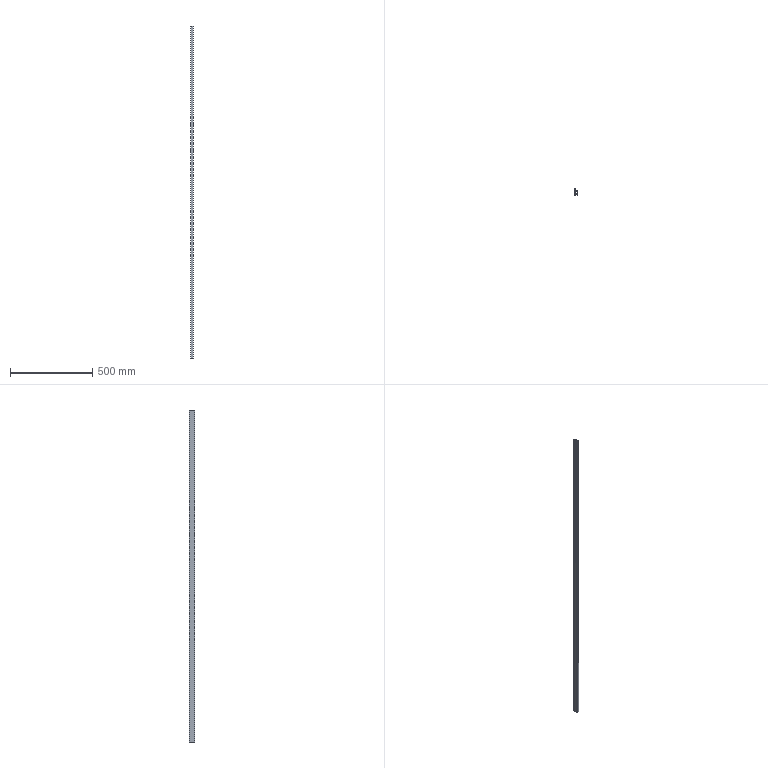Part | 1 solid | 40 faces | box 14.605 x 34.798 x 2016 mm | volume 327940 mm3 | plane 23 | cylinder 17 | commonest cylinder face diameters 0.24 x4 0.2 x3 0.4 x2 0.5 x2 1 x2 1.2 x2
STEP:
#1=CARTESIAN_POINT('',(5.7,32.998,1008.));
#2=VERTEX_POINT('',#1);
#3=CARTESIAN_POINT('',(5.8,32.898,1008.));
#4=VERTEX_POINT('',#3);
#5=CARTESIAN_POINT('',(5.8,32.998,1008.));
#6=DIRECTION('',(0.,0.,1.));
#7=DIRECTION('',(1.,0.,0.));
#8=AXIS2_PLACEMENT_3D('',#5,#6,#7);
#9=CIRCLE('',#8,0.1);
#10=EDGE_CURVE('',#2,#4,#9,.T.);
#11=ORIENTED_EDGE('',*,*,#10,.F.);
#12=CARTESIAN_POINT('',(5.7,32.998,-1008.));
#13=VERTEX_POINT('',#12);
#14=CARTESIAN_POINT('',(5.7,32.998,1008.));
#15=DIRECTION('',(0.,0.,-1.));
#16=VECTOR('',#15,1000.);
#17=LINE('',#14,#16);
#18=EDGE_CURVE('',#2,#13,#17,.T.);
#19=ORIENTED_EDGE('',*,*,#18,.T.);
#20=CARTESIAN_POINT('',(5.8,32.898,-1008.));
#21=VERTEX_POINT('',#20);
#22=CARTESIAN_POINT('',(5.8,32.998,-1008.));
#23=DIRECTION('',(0.,0.,1.));
#24=DIRECTION('',(1.,0.,0.));
#25=AXIS2_PLACEMENT_3D('',#22,#23,#24);
#26=CIRCLE('',#25,0.1);
#27=EDGE_CURVE('',#13,#21,#26,.T.);
#28=ORIENTED_EDGE('',*,*,#27,.T.);
#29=CARTESIAN_POINT('',(5.8,32.898,1008.));
#30=DIRECTION('',(0.,0.,-1.));
#31=VECTOR('',#30,1000.);
#32=LINE('',#29,#31);
#33=EDGE_CURVE('',#4,#21,#32,.T.);
#34=ORIENTED_EDGE('',*,*,#33,.F.);
#35=EDGE_LOOP('',(#11,#19,#28,#34));
#36=FACE_OUTER_BOUND('',#35,.T.);
#37=CARTESIAN_POINT('',(5.8,32.998,1008.));
#38=DIRECTION('',(0.,0.,-1.));
#39=DIRECTION('',(-1.,0.,0.));
#40=AXIS2_PLACEMENT_3D('',#37,#38,#39);
#41=CYLINDRICAL_SURFACE('',#40,0.1);
#42=ADVANCED_FACE('',(#36),#41,.T.);
#43=CARTESIAN_POINT('',(1.75,10.,1008.));
#44=VERTEX_POINT('',#43);
#45=CARTESIAN_POINT('',(2.,10.25,1008.));
#46=VERTEX_POINT('',#45);
#47=CARTESIAN_POINT('',(2.,10.,1008.));
#48=DIRECTION('',(0.,0.,-1.));
#49=DIRECTION('',(1.,0.,0.));
#50=AXIS2_PLACEMENT_3D('',#47,#48,#49);
#51=CIRCLE('',#50,0.25);
#52=EDGE_CURVE('',#44,#46,#51,.T.);
#53=ORIENTED_EDGE('',*,*,#52,.F.);
#54=CARTESIAN_POINT('',(1.75,10.,-1008.));
#55=VERTEX_POINT('',#54);
#56=CARTESIAN_POINT('',(1.75,10.,1008.));
#57=DIRECTION('',(0.,0.,-1.));
#58=VECTOR('',#57,1000.);
#59=LINE('',#56,#58);
#60=EDGE_CURVE('',#44,#55,#59,.T.);
#61=ORIENTED_EDGE('',*,*,#60,.T.);
#62=CARTESIAN_POINT('',(2.,10.25,-1008.));
#63=VERTEX_POINT('',#62);
#64=CARTESIAN_POINT('',(2.,10.,-1008.));
#65=DIRECTION('',(0.,0.,-1.));
#66=DIRECTION('',(1.,0.,0.));
#67=AXIS2_PLACEMENT_3D('',#64,#65,#66);
#68=CIRCLE('',#67,0.25);
#69=EDGE_CURVE('',#55,#63,#68,.T.);
#70=ORIENTED_EDGE('',*,*,#69,.T.);
#71=CARTESIAN_POINT('',(2.,10.25,1008.));
#72=DIRECTION('',(0.,0.,-1.));
#73=VECTOR('',#72,1000.);
#74=LINE('',#71,#73);
#75=EDGE_CURVE('',#46,#63,#74,.T.);
#76=ORIENTED_EDGE('',*,*,#75,.F.);
#77=EDGE_LOOP('',(#53,#61,#70,#76));
#78=FACE_OUTER_BOUND('',#77,.T.);
#79=CARTESIAN_POINT('',(2.,10.,1008.));
#80=DIRECTION('',(0.,0.,-1.));
#81=DIRECTION('',(-1.,0.,0.));
#82=AXIS2_PLACEMENT_3D('',#79,#80,#81);
#83=CYLINDRICAL_SURFACE('',#82,0.25);
#84=ADVANCED_FACE('',(#78),#83,.F.);
#85=CARTESIAN_POINT('',(14.605,7.029,-1008.));
#86=VERTEX_POINT('',#85);
#87=CARTESIAN_POINT('',(14.485,7.149,-1008.));
#88=VERTEX_POINT('',#87);
#89=CARTESIAN_POINT('',(14.485,7.029,-1008.));
#90=DIRECTION('',(0.,0.,1.));
#91=DIRECTION('',(1.,0.,0.));
#92=AXIS2_PLACEMENT_3D('',#89,#90,#91);
#93=CIRCLE('',#92,0.12);
#94=EDGE_CURVE('',#86,#88,#93,.T.);
#95=ORIENTED_EDGE('',*,*,#94,.T.);
#96=CARTESIAN_POINT('',(14.485,7.149,1008.));
#97=VERTEX_POINT('',#96);
#98=CARTESIAN_POINT('',(14.485,7.149,1008.));
#99=DIRECTION('',(0.,0.,-1.));
#100=VECTOR('',#99,1000.);
#101=LINE('',#98,#100);
#102=EDGE_CURVE('',#97,#88,#101,.T.);
#103=ORIENTED_EDGE('',*,*,#102,.F.);
#104=CARTESIAN_POINT('',(14.605,7.029,1008.));
#105=VERTEX_POINT('',#104);
#106=CARTESIAN_POINT('',(14.485,7.029,1008.));
#107=DIRECTION('',(0.,0.,1.));
#108=DIRECTION('',(1.,0.,0.));
#109=AXIS2_PLACEMENT_3D('',#106,#107,#108);
#110=CIRCLE('',#109,0.12);
#111=EDGE_CURVE('',#105,#97,#110,.T.);
#112=ORIENTED_EDGE('',*,*,#111,.F.);
#113=CARTESIAN_POINT('',(14.605,7.029,1008.));
#114=DIRECTION('',(0.,0.,-1.));
#115=VECTOR('',#114,1000.);
#116=LINE('',#113,#115);
#117=EDGE_CURVE('',#105,#86,#116,.T.);
#118=ORIENTED_EDGE('',*,*,#117,.T.);
#119=EDGE_LOOP('',(#95,#103,#112,#118));
#120=FACE_OUTER_BOUND('',#119,.T.);
#121=CARTESIAN_POINT('',(14.485,7.029,1008.));
#122=DIRECTION('',(0.,0.,-1.));
#123=DIRECTION('',(-1.,0.,0.));
#124=AXIS2_PLACEMENT_3D('',#121,#122,#123);
#125=CYLINDRICAL_SURFACE('',#124,0.12);
#126=ADVANCED_FACE('',(#120),#125,.T.);
#127=CARTESIAN_POINT('',(13.705,7.149,-1008.));
#128=VERTEX_POINT('',#127);
#129=CARTESIAN_POINT('',(14.485,7.149,-1008.));
#130=DIRECTION('',(-1.,0.,0.));
#131=VECTOR('',#130,1000.);
#132=LINE('',#129,#131);
#133=EDGE_CURVE('',#88,#128,#132,.T.);
#134=ORIENTED_EDGE('',*,*,#133,.T.);
#135=CARTESIAN_POINT('',(13.705,7.149,1008.));
#136=VERTEX_POINT('',#135);
#137=CARTESIAN_POINT('',(13.705,7.149,1008.));
#138=DIRECTION('',(0.,0.,-1.));
#139=VECTOR('',#138,1000.);
#140=LINE('',#137,#139);
#141=EDGE_CURVE('',#136,#128,#140,.T.);
#142=ORIENTED_EDGE('',*,*,#141,.F.);
#143=CARTESIAN_POINT('',(14.485,7.149,1008.));
#144=DIRECTION('',(-1.,0.,0.));
#145=VECTOR('',#144,1000.);
#146=LINE('',#143,#145);
#147=EDGE_CURVE('',#97,#136,#146,.T.);
#148=ORIENTED_EDGE('',*,*,#147,.F.);
#149=ORIENTED_EDGE('',*,*,#102,.T.);
#150=EDGE_LOOP('',(#134,#142,#148,#149));
#151=FACE_OUTER_BOUND('',#150,.T.);
#152=CARTESIAN_POINT('',(14.485,7.149,1008.));
#153=DIRECTION('',(0.,-1.,0.));
#154=DIRECTION('',(0.,0.,-1.));
#155=AXIS2_PLACEMENT_3D('',#152,#153,#154);
#156=PLANE('',#155);
#157=ADVANCED_FACE('',(#151),#156,.F.);
#158=CARTESIAN_POINT('',(13.105,6.549,-1008.));
#159=VERTEX_POINT('',#158);
#160=CARTESIAN_POINT('',(13.705,6.549,-1008.));
#161=DIRECTION('',(0.,0.,1.));
#162=DIRECTION('',(1.,0.,0.));
#163=AXIS2_PLACEMENT_3D('',#160,#161,#162);
#164=CIRCLE('',#163,0.6);
#165=EDGE_CURVE('',#128,#159,#164,.T.);
#166=ORIENTED_EDGE('',*,*,#165,.T.);
#167=CARTESIAN_POINT('',(13.105,6.549,1008.));
#168=VERTEX_POINT('',#167);
#169=CARTESIAN_POINT('',(13.105,6.549,1008.));
#170=DIRECTION('',(0.,0.,-1.));
#171=VECTOR('',#170,1000.);
#172=LINE('',#169,#171);
#173=EDGE_CURVE('',#168,#159,#172,.T.);
#174=ORIENTED_EDGE('',*,*,#173,.F.);
#175=CARTESIAN_POINT('',(13.705,6.549,1008.));
#176=DIRECTION('',(0.,0.,1.));
#177=DIRECTION('',(1.,0.,0.));
#178=AXIS2_PLACEMENT_3D('',#175,#176,#177);
#179=CIRCLE('',#178,0.6);
#180=EDGE_CURVE('',#136,#168,#179,.T.);
#181=ORIENTED_EDGE('',*,*,#180,.F.);
#182=ORIENTED_EDGE('',*,*,#141,.T.);
#183=EDGE_LOOP('',(#166,#174,#181,#182));
#184=FACE_OUTER_BOUND('',#183,.T.);
#185=CARTESIAN_POINT('',(13.705,6.549,1008.));
#186=DIRECTION('',(0.,0.,-1.));
#187=DIRECTION('',(-1.,0.,0.));
#188=AXIS2_PLACEMENT_3D('',#185,#186,#187);
#189=CYLINDRICAL_SURFACE('',#188,0.6);
#190=ADVANCED_FACE('',(#184),#189,.T.);
#191=CARTESIAN_POINT('',(13.105,2.27,-1008.));
#192=VERTEX_POINT('',#191);
#193=CARTESIAN_POINT('',(13.105,6.549,-1008.));
#194=DIRECTION('',(0.,-1.,0.));
#195=VECTOR('',#194,1000.);
#196=LINE('',#193,#195);
#197=EDGE_CURVE('',#159,#192,#196,.T.);
#198=ORIENTED_EDGE('',*,*,#197,.T.);
#199=CARTESIAN_POINT('',(13.105,2.27,1008.));
#200=VERTEX_POINT('',#199);
#201=CARTESIAN_POINT('',(13.105,2.27,1008.));
#202=DIRECTION('',(0.,0.,-1.));
#203=VECTOR('',#202,1000.);
#204=LINE('',#201,#203);
#205=EDGE_CURVE('',#200,#192,#204,.T.);
#206=ORIENTED_EDGE('',*,*,#205,.F.);
#207=CARTESIAN_POINT('',(13.105,6.549,1008.));
#208=DIRECTION('',(0.,-1.,0.));
#209=VECTOR('',#208,1000.);
#210=LINE('',#207,#209);
#211=EDGE_CURVE('',#168,#200,#210,.T.);
#212=ORIENTED_EDGE('',*,*,#211,.F.);
#213=ORIENTED_EDGE('',*,*,#173,.T.);
#214=EDGE_LOOP('',(#198,#206,#212,#213));
#215=FACE_OUTER_BOUND('',#214,.T.);
#216=CARTESIAN_POINT('',(13.105,6.549,1008.));
#217=DIRECTION('',(1.,0.,0.));
#218=DIRECTION('',(0.,0.,-1.));
#219=AXIS2_PLACEMENT_3D('',#216,#217,#218);
#220=PLANE('',#219);
#221=ADVANCED_FACE('',(#215),#220,.F.);
#222=CARTESIAN_POINT('',(12.985,2.15,-1008.));
#223=VERTEX_POINT('',#222);
#224=CARTESIAN_POINT('',(12.985,2.27,-1008.));
#225=DIRECTION('',(0.,0.,-1.));
#226=DIRECTION('',(1.,0.,0.));
#227=AXIS2_PLACEMENT_3D('',#224,#225,#226);
#228=CIRCLE('',#227,0.12);
#229=EDGE_CURVE('',#192,#223,#228,.T.);
#230=ORIENTED_EDGE('',*,*,#229,.T.);
#231=CARTESIAN_POINT('',(12.985,2.15,1008.));
#232=VERTEX_POINT('',#231);
#233=CARTESIAN_POINT('',(12.985,2.15,1008.));
#234=DIRECTION('',(0.,0.,-1.));
#235=VECTOR('',#234,1000.);
#236=LINE('',#233,#235);
#237=EDGE_CURVE('',#232,#223,#236,.T.);
#238=ORIENTED_EDGE('',*,*,#237,.F.);
#239=CARTESIAN_POINT('',(12.985,2.27,1008.));
#240=DIRECTION('',(0.,0.,-1.));
#241=DIRECTION('',(1.,0.,0.));
#242=AXIS2_PLACEMENT_3D('',#239,#240,#241);
#243=CIRCLE('',#242,0.12);
#244=EDGE_CURVE('',#200,#232,#243,.T.);
#245=ORIENTED_EDGE('',*,*,#244,.F.);
#246=ORIENTED_EDGE('',*,*,#205,.T.);
#247=EDGE_LOOP('',(#230,#238,#245,#246));
#248=FACE_OUTER_BOUND('',#247,.T.);
#249=CARTESIAN_POINT('',(12.985,2.27,1008.));
#250=DIRECTION('',(0.,0.,-1.));
#251=DIRECTION('',(-1.,0.,0.));
#252=AXIS2_PLACEMENT_3D('',#249,#250,#251);
#253=CYLINDRICAL_SURFACE('',#252,0.12);
#254=ADVANCED_FACE('',(#248),#253,.F.);
#255=CARTESIAN_POINT('',(2.5,2.15,-1008.));
#256=VERTEX_POINT('',#255);
#257=CARTESIAN_POINT('',(12.985,2.15,-1008.));
#258=DIRECTION('',(-1.,0.00001466,0.));
#259=VECTOR('',#258,1000.);
#260=LINE('',#257,#259);
#261=EDGE_CURVE('',#223,#256,#260,.T.);
#262=ORIENTED_EDGE('',*,*,#261,.T.);
#263=CARTESIAN_POINT('',(2.5,2.15,1008.));
#264=VERTEX_POINT('',#263);
#265=CARTESIAN_POINT('',(2.5,2.15,1008.));
#266=DIRECTION('',(0.,0.,-1.));
#267=VECTOR('',#266,1000.);
#268=LINE('',#265,#267);
#269=EDGE_CURVE('',#264,#256,#268,.T.);
#270=ORIENTED_EDGE('',*,*,#269,.F.);
#271=CARTESIAN_POINT('',(12.985,2.15,1008.));
#272=DIRECTION('',(-1.,0.00001466,0.));
#273=VECTOR('',#272,1000.);
#274=LINE('',#271,#273);
#275=EDGE_CURVE('',#232,#264,#274,.T.);
#276=ORIENTED_EDGE('',*,*,#275,.F.);
#277=ORIENTED_EDGE('',*,*,#237,.T.);
#278=EDGE_LOOP('',(#262,#270,#276,#277));
#279=FACE_OUTER_BOUND('',#278,.T.);
#280=CARTESIAN_POINT('',(12.985,2.15,1008.));
#281=DIRECTION('',(-0.00001466,-1.,0.));
#282=DIRECTION('',(1.,-0.00001466,0.));
#283=AXIS2_PLACEMENT_3D('',#280,#281,#282);
#284=PLANE('',#283);
#285=ADVANCED_FACE('',(#279),#284,.F.);
#286=CARTESIAN_POINT('',(2.,2.65,-1008.));
#287=VERTEX_POINT('',#286);
#288=CARTESIAN_POINT('',(2.5,2.65,-1008.));
#289=DIRECTION('',(0.,0.,-1.));
#290=DIRECTION('',(1.,0.,0.));
#291=AXIS2_PLACEMENT_3D('',#288,#289,#290);
#292=CIRCLE('',#291,0.5);
#293=EDGE_CURVE('',#256,#287,#292,.T.);
#294=ORIENTED_EDGE('',*,*,#293,.T.);
#295=CARTESIAN_POINT('',(2.,2.65,1008.));
#296=VERTEX_POINT('',#295);
#297=CARTESIAN_POINT('',(2.,2.65,1008.));
#298=DIRECTION('',(0.,0.,-1.));
#299=VECTOR('',#298,1000.);
#300=LINE('',#297,#299);
#301=EDGE_CURVE('',#296,#287,#300,.T.);
#302=ORIENTED_EDGE('',*,*,#301,.F.);
#303=CARTESIAN_POINT('',(2.5,2.65,1008.));
#304=DIRECTION('',(0.,0.,-1.));
#305=DIRECTION('',(1.,0.,0.));
#306=AXIS2_PLACEMENT_3D('',#303,#304,#305);
#307=CIRCLE('',#306,0.5);
#308=EDGE_CURVE('',#264,#296,#307,.T.);
#309=ORIENTED_EDGE('',*,*,#308,.F.);
#310=ORIENTED_EDGE('',*,*,#269,.T.);
#311=EDGE_LOOP('',(#294,#302,#309,#310));
#312=FACE_OUTER_BOUND('',#311,.T.);
#313=CARTESIAN_POINT('',(2.5,2.65,1008.));
#314=DIRECTION('',(0.,0.,-1.));
#315=DIRECTION('',(-1.,0.,0.));
#316=AXIS2_PLACEMENT_3D('',#313,#314,#315);
#317=CYLINDRICAL_SURFACE('',#316,0.5);
#318=ADVANCED_FACE('',(#312),#317,.F.);
#319=CARTESIAN_POINT('',(2.,9.75,-1008.));
#320=VERTEX_POINT('',#319);
#321=CARTESIAN_POINT('',(2.,2.65,-1008.));
#322=DIRECTION('',(0.,1.,0.));
#323=VECTOR('',#322,1000.);
#324=LINE('',#321,#323);
#325=EDGE_CURVE('',#287,#320,#324,.T.);
#326=ORIENTED_EDGE('',*,*,#325,.T.);
#327=CARTESIAN_POINT('',(2.,9.75,1008.));
#328=VERTEX_POINT('',#327);
#329=CARTESIAN_POINT('',(2.,9.75,1008.));
#330=DIRECTION('',(0.,0.,-1.));
#331=VECTOR('',#330,1000.);
#332=LINE('',#329,#331);
#333=EDGE_CURVE('',#328,#320,#332,.T.);
#334=ORIENTED_EDGE('',*,*,#333,.F.);
#335=CARTESIAN_POINT('',(2.,2.65,1008.));
#336=DIRECTION('',(0.,1.,0.));
#337=VECTOR('',#336,1000.);
#338=LINE('',#335,#337);
#339=EDGE_CURVE('',#296,#328,#338,.T.);
#340=ORIENTED_EDGE('',*,*,#339,.F.);
#341=ORIENTED_EDGE('',*,*,#301,.T.);
#342=EDGE_LOOP('',(#326,#334,#340,#341));
#343=FACE_OUTER_BOUND('',#342,.T.);
#344=CARTESIAN_POINT('',(2.,2.65,1008.));
#345=DIRECTION('',(-1.,0.,0.));
#346=DIRECTION('',(0.,0.,1.));
#347=AXIS2_PLACEMENT_3D('',#344,#345,#346);
#348=PLANE('',#347);
#349=ADVANCED_FACE('',(#343),#348,.F.);
#350=ORIENTED_EDGE('',*,*,#60,.F.);
#351=CARTESIAN_POINT('',(2.,10.,1008.));
#352=DIRECTION('',(0.,0.,-1.));
#353=DIRECTION('',(1.,0.,0.));
#354=AXIS2_PLACEMENT_3D('',#351,#352,#353);
#355=CIRCLE('',#354,0.25);
#356=EDGE_CURVE('',#328,#44,#355,.T.);
#357=ORIENTED_EDGE('',*,*,#356,.F.);
#358=ORIENTED_EDGE('',*,*,#333,.T.);
#359=CARTESIAN_POINT('',(2.,10.,-1008.));
#360=DIRECTION('',(0.,0.,-1.));
#361=DIRECTION('',(1.,0.,0.));
#362=AXIS2_PLACEMENT_3D('',#359,#360,#361);
#363=CIRCLE('',#362,0.25);
#364=EDGE_CURVE('',#320,#55,#363,.T.);
#365=ORIENTED_EDGE('',*,*,#364,.T.);
#366=EDGE_LOOP('',(#350,#357,#358,#365));
#367=FACE_OUTER_BOUND('',#366,.T.);
#368=CARTESIAN_POINT('',(2.,10.,1008.));
#369=DIRECTION('',(0.,0.,-1.));
#370=DIRECTION('',(-1.,0.,0.));
#371=AXIS2_PLACEMENT_3D('',#368,#369,#370);
#372=CYLINDRICAL_SURFACE('',#371,0.25);
#373=ADVANCED_FACE('',(#367),#372,.F.);
#374=CARTESIAN_POINT('',(2.,17.35,-1008.));
#375=VERTEX_POINT('',#374);
#376=CARTESIAN_POINT('',(2.,10.25,-1008.));
#377=DIRECTION('',(0.,1.,0.));
#378=VECTOR('',#377,1000.);
#379=LINE('',#376,#378);
#380=EDGE_CURVE('',#63,#375,#379,.T.);
#381=ORIENTED_EDGE('',*,*,#380,.T.);
#382=CARTESIAN_POINT('',(2.,17.35,1008.));
#383=VERTEX_POINT('',#382);
#384=CARTESIAN_POINT('',(2.,17.35,1008.));
#385=DIRECTION('',(0.,0.,-1.));
#386=VECTOR('',#385,1000.);
#387=LINE('',#384,#386);
#388=EDGE_CURVE('',#383,#375,#387,.T.);
#389=ORIENTED_EDGE('',*,*,#388,.F.);
#390=CARTESIAN_POINT('',(2.,10.25,1008.));
#391=DIRECTION('',(0.,1.,0.));
#392=VECTOR('',#391,1000.);
#393=LINE('',#390,#392);
#394=EDGE_CURVE('',#46,#383,#393,.T.);
#395=ORIENTED_EDGE('',*,*,#394,.F.);
#396=ORIENTED_EDGE('',*,*,#75,.T.);
#397=EDGE_LOOP('',(#381,#389,#395,#396));
#398=FACE_OUTER_BOUND('',#397,.T.);
#399=CARTESIAN_POINT('',(2.,10.25,1008.));
#400=DIRECTION('',(-1.,0.,0.));
#401=DIRECTION('',(0.,0.,1.));
#402=AXIS2_PLACEMENT_3D('',#399,#400,#401);
#403=PLANE('',#402);
#404=ADVANCED_FACE('',(#398),#403,.F.);
#405=CARTESIAN_POINT('',(2.5,17.85,-1008.));
#406=VERTEX_POINT('',#405);
#407=CARTESIAN_POINT('',(2.5,17.35,-1008.));
#408=DIRECTION('',(0.,0.,-1.));
#409=DIRECTION('',(1.,0.,0.));
#410=AXIS2_PLACEMENT_3D('',#407,#408,#409);
#411=CIRCLE('',#410,0.5);
#412=EDGE_CURVE('',#375,#406,#411,.T.);
#413=ORIENTED_EDGE('',*,*,#412,.T.);
#414=CARTESIAN_POINT('',(2.5,17.85,1008.));
#415=VERTEX_POINT('',#414);
#416=CARTESIAN_POINT('',(2.5,17.85,1008.));
#417=DIRECTION('',(0.,0.,-1.));
#418=VECTOR('',#417,1000.);
#419=LINE('',#416,#418);
#420=EDGE_CURVE('',#415,#406,#419,.T.);
#421=ORIENTED_EDGE('',*,*,#420,.F.);
#422=CARTESIAN_POINT('',(2.5,17.35,1008.));
#423=DIRECTION('',(0.,0.,-1.));
#424=DIRECTION('',(1.,0.,0.));
#425=AXIS2_PLACEMENT_3D('',#422,#423,#424);
#426=CIRCLE('',#425,0.5);
#427=EDGE_CURVE('',#383,#415,#426,.T.);
#428=ORIENTED_EDGE('',*,*,#427,.F.);
#429=ORIENTED_EDGE('',*,*,#388,.T.);
#430=EDGE_LOOP('',(#413,#421,#428,#429));
#431=FACE_OUTER_BOUND('',#430,.T.);
#432=CARTESIAN_POINT('',(2.5,17.35,1008.));
#433=DIRECTION('',(0.,0.,-1.));
#434=DIRECTION('',(-1.,0.,0.));
#435=AXIS2_PLACEMENT_3D('',#432,#433,#434);
#436=CYLINDRICAL_SURFACE('',#435,0.5);
#437=ADVANCED_FACE('',(#431),#436,.F.);
#438=CARTESIAN_POINT('',(14.604,17.85,-1008.));
#439=VERTEX_POINT('',#438);
#440=CARTESIAN_POINT('',(2.5,17.85,-1008.));
#441=DIRECTION('',(1.,0.,0.));
#442=VECTOR('',#441,1000.);
#443=LINE('',#440,#442);
#444=EDGE_CURVE('',#406,#439,#443,.T.);
#445=ORIENTED_EDGE('',*,*,#444,.T.);
#446=CARTESIAN_POINT('',(14.604,17.85,1008.));
#447=VERTEX_POINT('',#446);
#448=CARTESIAN_POINT('',(14.604,17.85,1008.));
#449=DIRECTION('',(0.,0.,-1.));
#450=VECTOR('',#449,1000.);
#451=LINE('',#448,#450);
#452=EDGE_CURVE('',#447,#439,#451,.T.);
#453=ORIENTED_EDGE('',*,*,#452,.F.);
#454=CARTESIAN_POINT('',(2.5,17.85,1008.));
#455=DIRECTION('',(1.,0.,0.));
#456=VECTOR('',#455,1000.);
#457=LINE('',#454,#456);
#458=EDGE_CURVE('',#415,#447,#457,.T.);
#459=ORIENTED_EDGE('',*,*,#458,.F.);
#460=ORIENTED_EDGE('',*,*,#420,.T.);
#461=EDGE_LOOP('',(#445,#453,#459,#460));
#462=FACE_OUTER_BOUND('',#461,.T.);
#463=CARTESIAN_POINT('',(2.5,17.85,1008.));
#464=DIRECTION('',(0.,1.,0.));
#465=DIRECTION('',(0.,0.,1.));
#466=AXIS2_PLACEMENT_3D('',#463,#464,#465);
#467=PLANE('',#466);
#468=ADVANCED_FACE('',(#462),#467,.F.);
#469=CARTESIAN_POINT('',(14.604,23.83,-1008.));
#470=VERTEX_POINT('',#469);
#471=CARTESIAN_POINT('',(14.604,17.85,-1008.));
#472=DIRECTION('',(0.,1.,0.));
#473=VECTOR('',#472,1000.);
#474=LINE('',#471,#473);
#475=EDGE_CURVE('',#439,#470,#474,.T.);
#476=ORIENTED_EDGE('',*,*,#475,.T.);
#477=CARTESIAN_POINT('',(14.604,23.83,1008.));
#478=VERTEX_POINT('',#477);
#479=CARTESIAN_POINT('',(14.604,23.83,1008.));
#480=DIRECTION('',(0.,0.,-1.));
#481=VECTOR('',#480,1000.);
#482=LINE('',#479,#481);
#483=EDGE_CURVE('',#478,#470,#482,.T.);
#484=ORIENTED_EDGE('',*,*,#483,.F.);
#485=CARTESIAN_POINT('',(14.604,17.85,1008.));
#486=DIRECTION('',(0.,1.,0.));
#487=VECTOR('',#486,1000.);
#488=LINE('',#485,#487);
#489=EDGE_CURVE('',#447,#478,#488,.T.);
#490=ORIENTED_EDGE('',*,*,#489,.F.);
#491=ORIENTED_EDGE('',*,*,#452,.T.);
#492=EDGE_LOOP('',(#476,#484,#490,#491));
#493=FACE_OUTER_BOUND('',#492,.T.);
#494=CARTESIAN_POINT('',(14.604,17.85,1008.));
#495=DIRECTION('',(-1.,0.,0.));
#496=DIRECTION('',(0.,0.,1.));
#497=AXIS2_PLACEMENT_3D('',#494,#495,#496);
#498=PLANE('',#497);
#499=ADVANCED_FACE('',(#493),#498,.F.);
#500=CARTESIAN_POINT('',(14.484,23.95,-1008.));
#501=VERTEX_POINT('',#500);
#502=CARTESIAN_POINT('',(14.484,23.83,-1008.));
#503=DIRECTION('',(0.,0.,1.));
#504=DIRECTION('',(1.,0.,0.));
#505=AXIS2_PLACEMENT_3D('',#502,#503,#504);
#506=CIRCLE('',#505,0.12);
#507=EDGE_CURVE('',#470,#501,#506,.T.);
#508=ORIENTED_EDGE('',*,*,#507,.T.);
#509=CARTESIAN_POINT('',(14.484,23.95,1008.));
#510=VERTEX_POINT('',#509);
#511=CARTESIAN_POINT('',(14.484,23.95,1008.));
#512=DIRECTION('',(0.,0.,-1.));
#513=VECTOR('',#512,1000.);
#514=LINE('',#511,#513);
#515=EDGE_CURVE('',#510,#501,#514,.T.);
#516=ORIENTED_EDGE('',*,*,#515,.F.);
#517=CARTESIAN_POINT('',(14.484,23.83,1008.));
#518=DIRECTION('',(0.,0.,1.));
#519=DIRECTION('',(1.,0.,0.));
#520=AXIS2_PLACEMENT_3D('',#517,#518,#519);
#521=CIRCLE('',#520,0.12);
#522=EDGE_CURVE('',#478,#510,#521,.T.);
#523=ORIENTED_EDGE('',*,*,#522,.F.);
#524=ORIENTED_EDGE('',*,*,#483,.T.);
#525=EDGE_LOOP('',(#508,#516,#523,#524));
#526=FACE_OUTER_BOUND('',#525,.T.);
#527=CARTESIAN_POINT('',(14.484,23.83,1008.));
#528=DIRECTION('',(0.,0.,-1.));
#529=DIRECTION('',(-1.,0.,0.));
#530=AXIS2_PLACEMENT_3D('',#527,#528,#529);
#531=CYLINDRICAL_SURFACE('',#530,0.12);
#532=ADVANCED_FACE('',(#526),#531,.T.);
#533=CARTESIAN_POINT('',(13.704,23.95,-1008.));
#534=VERTEX_POINT('',#533);
#535=CARTESIAN_POINT('',(14.484,23.95,-1008.));
#536=DIRECTION('',(-1.,0.,0.));
#537=VECTOR('',#536,1000.);
#538=LINE('',#535,#537);
#539=EDGE_CURVE('',#501,#534,#538,.T.);
#540=ORIENTED_EDGE('',*,*,#539,.T.);
#541=CARTESIAN_POINT('',(13.704,23.95,1008.));
#542=VERTEX_POINT('',#541);
#543=CARTESIAN_POINT('',(13.704,23.95,1008.));
#544=DIRECTION('',(0.,0.,-1.));
#545=VECTOR('',#544,1000.);
#546=LINE('',#543,#545);
#547=EDGE_CURVE('',#542,#534,#546,.T.);
#548=ORIENTED_EDGE('',*,*,#547,.F.);
#549=CARTESIAN_POINT('',(14.484,23.95,1008.));
#550=DIRECTION('',(-1.,0.,0.));
#551=VECTOR('',#550,1000.);
#552=LINE('',#549,#551);
#553=EDGE_CURVE('',#510,#542,#552,.T.);
#554=ORIENTED_EDGE('',*,*,#553,.F.);
#555=ORIENTED_EDGE('',*,*,#515,.T.);
#556=EDGE_LOOP('',(#540,#548,#554,#555));
#557=FACE_OUTER_BOUND('',#556,.T.);
#558=CARTESIAN_POINT('',(14.484,23.95,1008.));
#559=DIRECTION('',(0.,-1.,0.));
#560=DIRECTION('',(0.,0.,-1.));
#561=AXIS2_PLACEMENT_3D('',#558,#559,#560);
#562=PLANE('',#561);
#563=ADVANCED_FACE('',(#557),#562,.F.);
#564=CARTESIAN_POINT('',(13.104,23.35,-1008.));
#565=VERTEX_POINT('',#564);
#566=CARTESIAN_POINT('',(13.704,23.35,-1008.));
#567=DIRECTION('',(0.,0.,1.));
#568=DIRECTION('',(1.,0.,0.));
#569=AXIS2_PLACEMENT_3D('',#566,#567,#568);
#570=CIRCLE('',#569,0.6);
#571=EDGE_CURVE('',#534,#565,#570,.T.);
#572=ORIENTED_EDGE('',*,*,#571,.T.);
#573=CARTESIAN_POINT('',(13.104,23.35,1008.));
#574=VERTEX_POINT('',#573);
#575=CARTESIAN_POINT('',(13.104,23.35,1008.));
#576=DIRECTION('',(0.,0.,-1.));
#577=VECTOR('',#576,1000.);
#578=LINE('',#575,#577);
#579=EDGE_CURVE('',#574,#565,#578,.T.);
#580=ORIENTED_EDGE('',*,*,#579,.F.);
#581=CARTESIAN_POINT('',(13.704,23.35,1008.));
#582=DIRECTION('',(0.,0.,1.));
#583=DIRECTION('',(1.,0.,0.));
#584=AXIS2_PLACEMENT_3D('',#581,#582,#583);
#585=CIRCLE('',#584,0.6);
#586=EDGE_CURVE('',#542,#574,#585,.T.);
#587=ORIENTED_EDGE('',*,*,#586,.F.);
#588=ORIENTED_EDGE('',*,*,#547,.T.);
#589=EDGE_LOOP('',(#572,#580,#587,#588));
#590=FACE_OUTER_BOUND('',#589,.T.);
#591=CARTESIAN_POINT('',(13.704,23.35,1008.));
#592=DIRECTION('',(0.,0.,-1.));
#593=DIRECTION('',(-1.,0.,0.));
#594=AXIS2_PLACEMENT_3D('',#591,#592,#593);
#595=CYLINDRICAL_SURFACE('',#594,0.6);
#596=ADVANCED_FACE('',(#590),#595,.T.);
#597=CARTESIAN_POINT('',(13.104,19.47,-1008.));
#598=VERTEX_POINT('',#597);
#599=CARTESIAN_POINT('',(13.104,23.35,-1008.));
#600=DIRECTION('',(0.,-1.,0.));
#601=VECTOR('',#600,1000.);
#602=LINE('',#599,#601);
#603=EDGE_CURVE('',#565,#598,#602,.T.);
#604=ORIENTED_EDGE('',*,*,#603,.T.);
#605=CARTESIAN_POINT('',(13.104,19.47,1008.));
#606=VERTEX_POINT('',#605);
#607=CARTESIAN_POINT('',(13.104,19.47,1008.));
#608=DIRECTION('',(0.,0.,-1.));
#609=VECTOR('',#608,1000.);
#610=LINE('',#607,#609);
#611=EDGE_CURVE('',#606,#598,#610,.T.);
#612=ORIENTED_EDGE('',*,*,#611,.F.);
#613=CARTESIAN_POINT('',(13.104,23.35,1008.));
#614=DIRECTION('',(0.,-1.,0.));
#615=VECTOR('',#614,1000.);
#616=LINE('',#613,#615);
#617=EDGE_CURVE('',#574,#606,#616,.T.);
#618=ORIENTED_EDGE('',*,*,#617,.F.);
#619=ORIENTED_EDGE('',*,*,#579,.T.);
#620=EDGE_LOOP('',(#604,#612,#618,#619));
#621=FACE_OUTER_BOUND('',#620,.T.);
#622=CARTESIAN_POINT('',(13.104,23.35,1008.));
#623=DIRECTION('',(1.,0.,0.));
#624=DIRECTION('',(0.,0.,-1.));
#625=AXIS2_PLACEMENT_3D('',#622,#623,#624);
#626=PLANE('',#625);
#627=ADVANCED_FACE('',(#621),#626,.F.);
#628=CARTESIAN_POINT('',(12.984,19.35,-1008.));
#629=VERTEX_POINT('',#628);
#630=CARTESIAN_POINT('',(12.984,19.47,-1008.));
#631=DIRECTION('',(0.,0.,-1.));
#632=DIRECTION('',(1.,0.,0.));
#633=AXIS2_PLACEMENT_3D('',#630,#631,#632);
#634=CIRCLE('',#633,0.12);
#635=EDGE_CURVE('',#598,#629,#634,.T.);
#636=ORIENTED_EDGE('',*,*,#635,.T.);
#637=CARTESIAN_POINT('',(12.984,19.35,1008.));
#638=VERTEX_POINT('',#637);
#639=CARTESIAN_POINT('',(12.984,19.35,1008.));
#640=DIRECTION('',(0.,0.,-1.));
#641=VECTOR('',#640,1000.);
#642=LINE('',#639,#641);
#643=EDGE_CURVE('',#638,#629,#642,.T.);
#644=ORIENTED_EDGE('',*,*,#643,.F.);
#645=CARTESIAN_POINT('',(12.984,19.47,1008.));
#646=DIRECTION('',(0.,0.,-1.));
#647=DIRECTION('',(1.,0.,0.));
#648=AXIS2_PLACEMENT_3D('',#645,#646,#647);
#649=CIRCLE('',#648,0.12);
#650=EDGE_CURVE('',#606,#638,#649,.T.);
#651=ORIENTED_EDGE('',*,*,#650,.F.);
#652=ORIENTED_EDGE('',*,*,#611,.T.);
#653=EDGE_LOOP('',(#636,#644,#651,#652));
#654=FACE_OUTER_BOUND('',#653,.T.);
#655=CARTESIAN_POINT('',(12.984,19.47,1008.));
#656=DIRECTION('',(0.,0.,-1.));
#657=DIRECTION('',(-1.,0.,0.));
#658=AXIS2_PLACEMENT_3D('',#655,#656,#657);
#659=CYLINDRICAL_SURFACE('',#658,0.12);
#660=ADVANCED_FACE('',(#654),#659,.F.);
#661=CARTESIAN_POINT('',(7.2,19.35,-1008.));
#662=VERTEX_POINT('',#661);
#663=CARTESIAN_POINT('',(12.984,19.35,-1008.));
#664=DIRECTION('',(-1.,0.,0.));
#665=VECTOR('',#664,1000.);
#666=LINE('',#663,#665);
#667=EDGE_CURVE('',#629,#662,#666,.T.);
#668=ORIENTED_EDGE('',*,*,#667,.T.);
#669=CARTESIAN_POINT('',(7.2,19.35,1008.));
#670=VERTEX_POINT('',#669);
#671=CARTESIAN_POINT('',(7.2,19.35,1008.));
#672=DIRECTION('',(0.,0.,-1.));
#673=VECTOR('',#672,1000.);
#674=LINE('',#671,#673);
#675=EDGE_CURVE('',#670,#662,#674,.T.);
#676=ORIENTED_EDGE('',*,*,#675,.F.);
#677=CARTESIAN_POINT('',(12.984,19.35,1008.));
#678=DIRECTION('',(-1.,0.,0.));
#679=VECTOR('',#678,1000.);
#680=LINE('',#677,#679);
#681=EDGE_CURVE('',#638,#670,#680,.T.);
#682=ORIENTED_EDGE('',*,*,#681,.F.);
#683=ORIENTED_EDGE('',*,*,#643,.T.);
#684=EDGE_LOOP('',(#668,#676,#682,#683));
#685=FACE_OUTER_BOUND('',#684,.T.);
#686=CARTESIAN_POINT('',(12.984,19.35,1008.));
#687=DIRECTION('',(0.,-1.,0.));
#688=DIRECTION('',(0.,0.,-1.));
#689=AXIS2_PLACEMENT_3D('',#686,#687,#688);
#690=PLANE('',#689);
#691=ADVANCED_FACE('',(#685),#690,.F.);
#692=CARTESIAN_POINT('',(7.2,34.798,-1008.));
#693=VERTEX_POINT('',#692);
#694=CARTESIAN_POINT('',(7.2,19.35,-1008.));
#695=DIRECTION('',(0.,1.,0.));
#696=VECTOR('',#695,1000.);
#697=LINE('',#694,#696);
#698=EDGE_CURVE('',#662,#693,#697,.T.);
#699=ORIENTED_EDGE('',*,*,#698,.T.);
#700=CARTESIAN_POINT('',(7.2,34.798,1008.));
#701=VERTEX_POINT('',#700);
#702=CARTESIAN_POINT('',(7.2,34.798,1008.));
#703=DIRECTION('',(0.,0.,-1.));
#704=VECTOR('',#703,1000.);
#705=LINE('',#702,#704);
#706=EDGE_CURVE('',#701,#693,#705,.T.);
#707=ORIENTED_EDGE('',*,*,#706,.F.);
#708=CARTESIAN_POINT('',(7.2,19.35,1008.));
#709=DIRECTION('',(0.,1.,0.));
#710=VECTOR('',#709,1000.);
#711=LINE('',#708,#710);
#712=EDGE_CURVE('',#670,#701,#711,.T.);
#713=ORIENTED_EDGE('',*,*,#712,.F.);
#714=ORIENTED_EDGE('',*,*,#675,.T.);
#715=EDGE_LOOP('',(#699,#707,#713,#714));
#716=FACE_OUTER_BOUND('',#715,.T.);
#717=CARTESIAN_POINT('',(7.2,19.35,1008.));
#718=DIRECTION('',(-1.,0.,0.));
#719=DIRECTION('',(0.,0.,1.));
#720=AXIS2_PLACEMENT_3D('',#717,#718,#719);
#721=PLANE('',#720);
#722=ADVANCED_FACE('',(#716),#721,.F.);
#723=CARTESIAN_POINT('',(6.,34.798,-1008.));
#724=VERTEX_POINT('',#723);
#725=CARTESIAN_POINT('',(7.2,34.798,-1008.));
#726=DIRECTION('',(-1.,0.,0.));
#727=VECTOR('',#726,1000.);
#728=LINE('',#725,#727);
#729=EDGE_CURVE('',#693,#724,#728,.T.);
#730=ORIENTED_EDGE('',*,*,#729,.T.);
#731=CARTESIAN_POINT('',(6.,34.798,1008.));
#732=VERTEX_POINT('',#731);
#733=CARTESIAN_POINT('',(6.,34.798,1008.));
#734=DIRECTION('',(0.,0.,-1.));
#735=VECTOR('',#734,1000.);
#736=LINE('',#733,#735);
#737=EDGE_CURVE('',#732,#724,#736,.T.);
#738=ORIENTED_EDGE('',*,*,#737,.F.);
#739=CARTESIAN_POINT('',(7.2,34.798,1008.));
#740=DIRECTION('',(-1.,0.,0.));
#741=VECTOR('',#740,1000.);
#742=LINE('',#739,#741);
#743=EDGE_CURVE('',#701,#732,#742,.T.);
#744=ORIENTED_EDGE('',*,*,#743,.F.);
#745=ORIENTED_EDGE('',*,*,#706,.T.);
#746=EDGE_LOOP('',(#730,#738,#744,#745));
#747=FACE_OUTER_BOUND('',#746,.T.);
#748=CARTESIAN_POINT('',(7.2,34.798,1008.));
#749=DIRECTION('',(0.,-1.,0.));
#750=DIRECTION('',(0.,0.,-1.));
#751=AXIS2_PLACEMENT_3D('',#748,#749,#750);
#752=PLANE('',#751);
#753=ADVANCED_FACE('',(#747),#752,.F.);
#754=CARTESIAN_POINT('',(5.8,34.598,-1008.));
#755=VERTEX_POINT('',#754);
#756=CARTESIAN_POINT('',(6.,34.598,-1008.));
#757=DIRECTION('',(0.,0.,1.));
#758=DIRECTION('',(1.,0.,0.));
#759=AXIS2_PLACEMENT_3D('',#756,#757,#758);
#760=CIRCLE('',#759,0.2);
#761=EDGE_CURVE('',#724,#755,#760,.T.);
#762=ORIENTED_EDGE('',*,*,#761,.T.);
#763=CARTESIAN_POINT('',(5.8,34.598,1008.));
#764=VERTEX_POINT('',#763);
#765=CARTESIAN_POINT('',(5.8,34.598,1008.));
#766=DIRECTION('',(0.,0.,-1.));
#767=VECTOR('',#766,1000.);
#768=LINE('',#765,#767);
#769=EDGE_CURVE('',#764,#755,#768,.T.);
#770=ORIENTED_EDGE('',*,*,#769,.F.);
#771=CARTESIAN_POINT('',(6.,34.598,1008.));
#772=DIRECTION('',(0.,0.,1.));
#773=DIRECTION('',(1.,0.,0.));
#774=AXIS2_PLACEMENT_3D('',#771,#772,#773);
#775=CIRCLE('',#774,0.2);
#776=EDGE_CURVE('',#732,#764,#775,.T.);
#777=ORIENTED_EDGE('',*,*,#776,.F.);
#778=ORIENTED_EDGE('',*,*,#737,.T.);
#779=EDGE_LOOP('',(#762,#770,#777,#778));
#780=FACE_OUTER_BOUND('',#779,.T.);
#781=CARTESIAN_POINT('',(6.,34.598,1008.));
#782=DIRECTION('',(0.,0.,-1.));
#783=DIRECTION('',(-1.,0.,0.));
#784=AXIS2_PLACEMENT_3D('',#781,#782,#783);
#785=CYLINDRICAL_SURFACE('',#784,0.2);
#786=ADVANCED_FACE('',(#780),#785,.T.);
#787=CARTESIAN_POINT('',(5.8,33.098,-1008.));
#788=VERTEX_POINT('',#787);
#789=CARTESIAN_POINT('',(5.8,34.598,-1008.));
#790=DIRECTION('',(0.,-1.,0.));
#791=VECTOR('',#790,1000.);
#792=LINE('',#789,#791);
#793=EDGE_CURVE('',#755,#788,#792,.T.);
#794=ORIENTED_EDGE('',*,*,#793,.T.);
#795=CARTESIAN_POINT('',(5.8,33.098,1008.));
#796=VERTEX_POINT('',#795);
#797=CARTESIAN_POINT('',(5.8,33.098,1008.));
#798=DIRECTION('',(0.,0.,-1.));
#799=VECTOR('',#798,1000.);
#800=LINE('',#797,#799);
#801=EDGE_CURVE('',#796,#788,#800,.T.);
#802=ORIENTED_EDGE('',*,*,#801,.F.);
#803=CARTESIAN_POINT('',(5.8,34.598,1008.));
#804=DIRECTION('',(0.,-1.,0.));
#805=VECTOR('',#804,1000.);
#806=LINE('',#803,#805);
#807=EDGE_CURVE('',#764,#796,#806,.T.);
#808=ORIENTED_EDGE('',*,*,#807,.F.);
#809=ORIENTED_EDGE('',*,*,#769,.T.);
#810=EDGE_LOOP('',(#794,#802,#808,#809));
#811=FACE_OUTER_BOUND('',#810,.T.);
#812=CARTESIAN_POINT('',(5.8,34.598,1008.));
#813=DIRECTION('',(1.,0.,0.));
#814=DIRECTION('',(0.,0.,-1.));
#815=AXIS2_PLACEMENT_3D('',#812,#813,#814);
#816=PLANE('',#815);
#817=ADVANCED_FACE('',(#811),#816,.F.);
#818=ORIENTED_EDGE('',*,*,#18,.F.);
#819=CARTESIAN_POINT('',(5.8,32.998,1008.));
#820=DIRECTION('',(0.,0.,1.));
#821=DIRECTION('',(1.,0.,0.));
#822=AXIS2_PLACEMENT_3D('',#819,#820,#821);
#823=CIRCLE('',#822,0.1);
#824=EDGE_CURVE('',#796,#2,#823,.T.);
#825=ORIENTED_EDGE('',*,*,#824,.F.);
#826=ORIENTED_EDGE('',*,*,#801,.T.);
#827=CARTESIAN_POINT('',(5.8,32.998,-1008.));
#828=DIRECTION('',(0.,0.,1.));
#829=DIRECTION('',(1.,0.,0.));
#830=AXIS2_PLACEMENT_3D('',#827,#828,#829);
#831=CIRCLE('',#830,0.1);
#832=EDGE_CURVE('',#788,#13,#831,.T.);
#833=ORIENTED_EDGE('',*,*,#832,.T.);
#834=EDGE_LOOP('',(#818,#825,#826,#833));
#835=FACE_OUTER_BOUND('',#834,.T.);
#836=CARTESIAN_POINT('',(5.8,32.998,1008.));
#837=DIRECTION('',(0.,0.,-1.));
#838=DIRECTION('',(-1.,0.,0.));
#839=AXIS2_PLACEMENT_3D('',#836,#837,#838);
#840=CYLINDRICAL_SURFACE('',#839,0.1);
#841=ADVANCED_FACE('',(#835),#840,.T.);
#842=CARTESIAN_POINT('',(5.8,23.812,-1008.));
#843=VERTEX_POINT('',#842);
#844=CARTESIAN_POINT('',(5.8,32.898,-1008.));
#845=DIRECTION('',(0.,-1.,0.));
#846=VECTOR('',#845,1000.);
#847=LINE('',#844,#846);
#848=EDGE_CURVE('',#21,#843,#847,.T.);
#849=ORIENTED_EDGE('',*,*,#848,.T.);
#850=CARTESIAN_POINT('',(5.8,23.812,1008.));
#851=VERTEX_POINT('',#850);
#852=CARTESIAN_POINT('',(5.8,23.812,1008.));
#853=DIRECTION('',(0.,0.,-1.));
#854=VECTOR('',#853,1000.);
#855=LINE('',#852,#854);
#856=EDGE_CURVE('',#851,#843,#855,.T.);
#857=ORIENTED_EDGE('',*,*,#856,.F.);
#858=CARTESIAN_POINT('',(5.8,32.898,1008.));
#859=DIRECTION('',(0.,-1.,0.));
#860=VECTOR('',#859,1000.);
#861=LINE('',#858,#860);
#862=EDGE_CURVE('',#4,#851,#861,.T.);
#863=ORIENTED_EDGE('',*,*,#862,.F.);
#864=ORIENTED_EDGE('',*,*,#33,.T.);
#865=EDGE_LOOP('',(#849,#857,#863,#864));
#866=FACE_OUTER_BOUND('',#865,.T.);
#867=CARTESIAN_POINT('',(5.8,32.898,1008.));
#868=DIRECTION('',(1.,0.,0.));
#869=DIRECTION('',(0.,0.,-1.));
#870=AXIS2_PLACEMENT_3D('',#867,#868,#869);
#871=PLANE('',#870);
#872=ADVANCED_FACE('',(#866),#871,.F.);
#873=CARTESIAN_POINT('',(4.8,22.812,-1008.));
#874=VERTEX_POINT('',#873);
#875=CARTESIAN_POINT('',(4.8,23.812,-1008.));
#876=DIRECTION('',(0.,0.,-1.));
#877=DIRECTION('',(1.,0.,0.));
#878=AXIS2_PLACEMENT_3D('',#875,#876,#877);
#879=CIRCLE('',#878,1.);
#880=EDGE_CURVE('',#843,#874,#879,.T.);
#881=ORIENTED_EDGE('',*,*,#880,.T.);
#882=CARTESIAN_POINT('',(4.8,22.812,1008.));
#883=VERTEX_POINT('',#882);
#884=CARTESIAN_POINT('',(4.8,22.812,1008.));
#885=DIRECTION('',(0.,0.,-1.));
#886=VECTOR('',#885,1000.);
#887=LINE('',#884,#886);
#888=EDGE_CURVE('',#883,#874,#887,.T.);
#889=ORIENTED_EDGE('',*,*,#888,.F.);
#890=CARTESIAN_POINT('',(4.8,23.812,1008.));
#891=DIRECTION('',(0.,0.,-1.));
#892=DIRECTION('',(1.,0.,0.));
#893=AXIS2_PLACEMENT_3D('',#890,#891,#892);
#894=CIRCLE('',#893,1.);
#895=EDGE_CURVE('',#851,#883,#894,.T.);
#896=ORIENTED_EDGE('',*,*,#895,.F.);
#897=ORIENTED_EDGE('',*,*,#856,.T.);
#898=EDGE_LOOP('',(#881,#889,#896,#897));
#899=FACE_OUTER_BOUND('',#898,.T.);
#900=CARTESIAN_POINT('',(4.8,23.812,1008.));
#901=DIRECTION('',(0.,0.,-1.));
#902=DIRECTION('',(-1.,0.,0.));
#903=AXIS2_PLACEMENT_3D('',#900,#901,#902);
#904=CYLINDRICAL_SURFACE('',#903,1.);
#905=ADVANCED_FACE('',(#899),#904,.F.);
#906=CARTESIAN_POINT('',(2.8,22.812,-1008.));
#907=VERTEX_POINT('',#906);
#908=CARTESIAN_POINT('',(4.8,22.812,-1008.));
#909=DIRECTION('',(-1.,0.,0.));
#910=VECTOR('',#909,1000.);
#911=LINE('',#908,#910);
#912=EDGE_CURVE('',#874,#907,#911,.T.);
#913=ORIENTED_EDGE('',*,*,#912,.T.);
#914=CARTESIAN_POINT('',(2.8,22.812,1008.));
#915=VERTEX_POINT('',#914);
#916=CARTESIAN_POINT('',(2.8,22.812,1008.));
#917=DIRECTION('',(0.,0.,-1.));
#918=VECTOR('',#917,1000.);
#919=LINE('',#916,#918);
#920=EDGE_CURVE('',#915,#907,#919,.T.);
#921=ORIENTED_EDGE('',*,*,#920,.F.);
#922=CARTESIAN_POINT('',(4.8,22.812,1008.));
#923=DIRECTION('',(-1.,0.,0.));
#924=VECTOR('',#923,1000.);
#925=LINE('',#922,#924);
#926=EDGE_CURVE('',#883,#915,#925,.T.);
#927=ORIENTED_EDGE('',*,*,#926,.F.);
#928=ORIENTED_EDGE('',*,*,#888,.T.);
#929=EDGE_LOOP('',(#913,#921,#927,#928));
#930=FACE_OUTER_BOUND('',#929,.T.);
#931=CARTESIAN_POINT('',(4.8,22.812,1008.));
#932=DIRECTION('',(0.,-1.,0.));
#933=DIRECTION('',(0.,0.,-1.));
#934=AXIS2_PLACEMENT_3D('',#931,#932,#933);
#935=PLANE('',#934);
#936=ADVANCED_FACE('',(#930),#935,.F.);
#937=CARTESIAN_POINT('',(1.8,23.812,-1008.));
#938=VERTEX_POINT('',#937);
#939=CARTESIAN_POINT('',(2.8,23.812,-1008.));
#940=DIRECTION('',(0.,0.,-1.));
#941=DIRECTION('',(1.,0.,0.));
#942=AXIS2_PLACEMENT_3D('',#939,#940,#941);
#943=CIRCLE('',#942,1.);
#944=EDGE_CURVE('',#907,#938,#943,.T.);
#945=ORIENTED_EDGE('',*,*,#944,.T.);
#946=CARTESIAN_POINT('',(1.8,23.812,1008.));
#947=VERTEX_POINT('',#946);
#948=CARTESIAN_POINT('',(1.8,23.812,1008.));
#949=DIRECTION('',(0.,0.,-1.));
#950=VECTOR('',#949,1000.);
#951=LINE('',#948,#950);
#952=EDGE_CURVE('',#947,#938,#951,.T.);
#953=ORIENTED_EDGE('',*,*,#952,.F.);
#954=CARTESIAN_POINT('',(2.8,23.812,1008.));
#955=DIRECTION('',(0.,0.,-1.));
#956=DIRECTION('',(1.,0.,0.));
#957=AXIS2_PLACEMENT_3D('',#954,#955,#956);
#958=CIRCLE('',#957,1.);
#959=EDGE_CURVE('',#915,#947,#958,.T.);
#960=ORIENTED_EDGE('',*,*,#959,.F.);
#961=ORIENTED_EDGE('',*,*,#920,.T.);
#962=EDGE_LOOP('',(#945,#953,#960,#961));
#963=FACE_OUTER_BOUND('',#962,.T.);
#964=CARTESIAN_POINT('',(2.8,23.812,1008.));
#965=DIRECTION('',(0.,0.,-1.));
#966=DIRECTION('',(-1.,0.,0.));
#967=AXIS2_PLACEMENT_3D('',#964,#965,#966);
#968=CYLINDRICAL_SURFACE('',#967,1.);
#969=ADVANCED_FACE('',(#963),#968,.F.);
#970=CARTESIAN_POINT('',(1.8,32.898,-1008.));
#971=VERTEX_POINT('',#970);
#972=CARTESIAN_POINT('',(1.8,23.812,-1008.));
#973=DIRECTION('',(0.,1.,0.));
#974=VECTOR('',#973,1000.);
#975=LINE('',#972,#974);
#976=EDGE_CURVE('',#938,#971,#975,.T.);
#977=ORIENTED_EDGE('',*,*,#976,.T.);
#978=CARTESIAN_POINT('',(1.8,32.898,1008.));
#979=VERTEX_POINT('',#978);
#980=CARTESIAN_POINT('',(1.8,32.898,1008.));
#981=DIRECTION('',(0.,0.,-1.));
#982=VECTOR('',#981,1000.);
#983=LINE('',#980,#982);
#984=EDGE_CURVE('',#979,#971,#983,.T.);
#985=ORIENTED_EDGE('',*,*,#984,.F.);
#986=CARTESIAN_POINT('',(1.8,23.812,1008.));
#987=DIRECTION('',(0.,1.,0.));
#988=VECTOR('',#987,1000.);
#989=LINE('',#986,#988);
#990=EDGE_CURVE('',#947,#979,#989,.T.);
#991=ORIENTED_EDGE('',*,*,#990,.F.);
#992=ORIENTED_EDGE('',*,*,#952,.T.);
#993=EDGE_LOOP('',(#977,#985,#991,#992));
#994=FACE_OUTER_BOUND('',#993,.T.);
#995=CARTESIAN_POINT('',(1.8,23.812,1008.));
#996=DIRECTION('',(-1.,0.,0.));
#997=DIRECTION('',(0.,0.,1.));
#998=AXIS2_PLACEMENT_3D('',#995,#996,#997);
#999=PLANE('',#998);
#1000=ADVANCED_FACE('',(#994),#999,.F.);
#1001=CARTESIAN_POINT('',(1.8,33.098,-1008.));
#1002=VERTEX_POINT('',#1001);
#1003=CARTESIAN_POINT('',(1.8,32.998,-1008.));
#1004=DIRECTION('',(0.,0.,1.));
#1005=DIRECTION('',(1.,0.,0.));
#1006=AXIS2_PLACEMENT_3D('',#1003,#1004,#1005);
#1007=CIRCLE('',#1006,0.1);
#1008=EDGE_CURVE('',#971,#1002,#1007,.T.);
#1009=ORIENTED_EDGE('',*,*,#1008,.T.);
#1010=CARTESIAN_POINT('',(1.8,33.098,1008.));
#1011=VERTEX_POINT('',#1010);
#1012=CARTESIAN_POINT('',(1.8,33.098,1008.));
#1013=DIRECTION('',(0.,0.,-1.));
#1014=VECTOR('',#1013,1000.);
#1015=LINE('',#1012,#1014);
#1016=EDGE_CURVE('',#1011,#1002,#1015,.T.);
#1017=ORIENTED_EDGE('',*,*,#1016,.F.);
#1018=CARTESIAN_POINT('',(1.8,32.998,1008.));
#1019=DIRECTION('',(0.,0.,1.));
#1020=DIRECTION('',(1.,0.,0.));
#1021=AXIS2_PLACEMENT_3D('',#1018,#1019,#1020);
#1022=CIRCLE('',#1021,0.1);
#1023=EDGE_CURVE('',#979,#1011,#1022,.T.);
#1024=ORIENTED_EDGE('',*,*,#1023,.F.);
#1025=ORIENTED_EDGE('',*,*,#984,.T.);
#1026=EDGE_LOOP('',(#1009,#1017,#1024,#1025));
#1027=FACE_OUTER_BOUND('',#1026,.T.);
#1028=CARTESIAN_POINT('',(1.8,32.998,1008.));
#1029=DIRECTION('',(0.,0.,-1.));
#1030=DIRECTION('',(-1.,0.,0.));
#1031=AXIS2_PLACEMENT_3D('',#1028,#1029,#1030);
#1032=CYLINDRICAL_SURFACE('',#1031,0.1);
#1033=ADVANCED_FACE('',(#1027),#1032,.T.);
#1034=CARTESIAN_POINT('',(1.8,34.598,-1008.));
#1035=VERTEX_POINT('',#1034);
#1036=CARTESIAN_POINT('',(1.8,33.098,-1008.));
#1037=DIRECTION('',(0.,1.,0.));
#1038=VECTOR('',#1037,1000.);
#1039=LINE('',#1036,#1038);
#1040=EDGE_CURVE('',#1002,#1035,#1039,.T.);
#1041=ORIENTED_EDGE('',*,*,#1040,.T.);
#1042=CARTESIAN_POINT('',(1.8,34.598,1008.));
#1043=VERTEX_POINT('',#1042);
#1044=CARTESIAN_POINT('',(1.8,34.598,1008.));
#1045=DIRECTION('',(0.,0.,-1.));
#1046=VECTOR('',#1045,1000.);
#1047=LINE('',#1044,#1046);
#1048=EDGE_CURVE('',#1043,#1035,#1047,.T.);
#1049=ORIENTED_EDGE('',*,*,#1048,.F.);
#1050=CARTESIAN_POINT('',(1.8,33.098,1008.));
#1051=DIRECTION('',(0.,1.,0.));
#1052=VECTOR('',#1051,1000.);
#1053=LINE('',#1050,#1052);
#1054=EDGE_CURVE('',#1011,#1043,#1053,.T.);
#1055=ORIENTED_EDGE('',*,*,#1054,.F.);
#1056=ORIENTED_EDGE('',*,*,#1016,.T.);
#1057=EDGE_LOOP('',(#1041,#1049,#1055,#1056));
#1058=FACE_OUTER_BOUND('',#1057,.T.);
#1059=CARTESIAN_POINT('',(1.8,33.098,1008.));
#1060=DIRECTION('',(-1.,0.,0.));
#1061=DIRECTION('',(0.,0.,1.));
#1062=AXIS2_PLACEMENT_3D('',#1059,#1060,#1061);
#1063=PLANE('',#1062);
#1064=ADVANCED_FACE('',(#1058),#1063,.F.);
#1065=CARTESIAN_POINT('',(1.6,34.798,-1008.));
#1066=VERTEX_POINT('',#1065);
#1067=CARTESIAN_POINT('',(1.6,34.598,-1008.));
#1068=DIRECTION('',(0.,0.,1.));
#1069=DIRECTION('',(1.,0.,0.));
#1070=AXIS2_PLACEMENT_3D('',#1067,#1068,#1069);
#1071=CIRCLE('',#1070,0.2);
#1072=EDGE_CURVE('',#1035,#1066,#1071,.T.);
#1073=ORIENTED_EDGE('',*,*,#1072,.T.);
#1074=CARTESIAN_POINT('',(1.6,34.798,1008.));
#1075=VERTEX_POINT('',#1074);
#1076=CARTESIAN_POINT('',(1.6,34.798,1008.));
#1077=DIRECTION('',(0.,0.,-1.));
#1078=VECTOR('',#1077,1000.);
#1079=LINE('',#1076,#1078);
#1080=EDGE_CURVE('',#1075,#1066,#1079,.T.);
#1081=ORIENTED_EDGE('',*,*,#1080,.F.);
#1082=CARTESIAN_POINT('',(1.6,34.598,1008.));
#1083=DIRECTION('',(0.,0.,1.));
#1084=DIRECTION('',(1.,0.,0.));
#1085=AXIS2_PLACEMENT_3D('',#1082,#1083,#1084);
#1086=CIRCLE('',#1085,0.2);
#1087=EDGE_CURVE('',#1043,#1075,#1086,.T.);
#1088=ORIENTED_EDGE('',*,*,#1087,.F.);
#1089=ORIENTED_EDGE('',*,*,#1048,.T.);
#1090=EDGE_LOOP('',(#1073,#1081,#1088,#1089));
#1091=FACE_OUTER_BOUND('',#1090,.T.);
#1092=CARTESIAN_POINT('',(1.6,34.598,1008.));
#1093=DIRECTION('',(0.,0.,-1.));
#1094=DIRECTION('',(-1.,0.,0.));
#1095=AXIS2_PLACEMENT_3D('',#1092,#1093,#1094);
#1096=CYLINDRICAL_SURFACE('',#1095,0.2);
#1097=ADVANCED_FACE('',(#1091),#1096,.T.);
#1098=CARTESIAN_POINT('',(0.,34.798,-1008.));
#1099=VERTEX_POINT('',#1098);
#1100=CARTESIAN_POINT('',(1.6,34.798,-1008.));
#1101=DIRECTION('',(-1.,0.,0.));
#1102=VECTOR('',#1101,1000.);
#1103=LINE('',#1100,#1102);
#1104=EDGE_CURVE('',#1066,#1099,#1103,.T.);
#1105=ORIENTED_EDGE('',*,*,#1104,.T.);
#1106=CARTESIAN_POINT('',(0.,34.798,1008.));
#1107=VERTEX_POINT('',#1106);
#1108=CARTESIAN_POINT('',(0.,34.798,1008.));
#1109=DIRECTION('',(0.,0.,-1.));
#1110=VECTOR('',#1109,1000.);
#1111=LINE('',#1108,#1110);
#1112=EDGE_CURVE('',#1107,#1099,#1111,.T.);
#1113=ORIENTED_EDGE('',*,*,#1112,.F.);
#1114=CARTESIAN_POINT('',(1.6,34.798,1008.));
#1115=DIRECTION('',(-1.,0.,0.));
#1116=VECTOR('',#1115,1000.);
#1117=LINE('',#1114,#1116);
#1118=EDGE_CURVE('',#1075,#1107,#1117,.T.);
#1119=ORIENTED_EDGE('',*,*,#1118,.F.);
#1120=ORIENTED_EDGE('',*,*,#1080,.T.);
#1121=EDGE_LOOP('',(#1105,#1113,#1119,#1120));
#1122=FACE_OUTER_BOUND('',#1121,.T.);
#1123=CARTESIAN_POINT('',(1.6,34.798,1008.));
#1124=DIRECTION('',(0.,-1.,0.));
#1125=DIRECTION('',(0.,0.,-1.));
#1126=AXIS2_PLACEMENT_3D('',#1123,#1124,#1125);
#1127=PLANE('',#1126);
#1128=ADVANCED_FACE('',(#1122),#1127,.F.);
#1129=CARTESIAN_POINT('',(0.,0.,-1008.));
#1130=VERTEX_POINT('',#1129);
#1131=CARTESIAN_POINT('',(0.,34.798,-1008.));
#1132=DIRECTION('',(0.,-1.,0.));
#1133=VECTOR('',#1132,1000.);
#1134=LINE('',#1131,#1133);
#1135=EDGE_CURVE('',#1099,#1130,#1134,.T.);
#1136=ORIENTED_EDGE('',*,*,#1135,.T.);
#1137=CARTESIAN_POINT('',(0.,0.,1008.));
#1138=VERTEX_POINT('',#1137);
#1139=CARTESIAN_POINT('',(0.,0.,1008.));
#1140=DIRECTION('',(0.,0.,-1.));
#1141=VECTOR('',#1140,1000.);
#1142=LINE('',#1139,#1141);
#1143=EDGE_CURVE('',#1138,#1130,#1142,.T.);
#1144=ORIENTED_EDGE('',*,*,#1143,.F.);
#1145=CARTESIAN_POINT('',(0.,34.798,1008.));
#1146=DIRECTION('',(0.,-1.,0.));
#1147=VECTOR('',#1146,1000.);
#1148=LINE('',#1145,#1147);
#1149=EDGE_CURVE('',#1107,#1138,#1148,.T.);
#1150=ORIENTED_EDGE('',*,*,#1149,.F.);
#1151=ORIENTED_EDGE('',*,*,#1112,.T.);
#1152=EDGE_LOOP('',(#1136,#1144,#1150,#1151));
#1153=FACE_OUTER_BOUND('',#1152,.T.);
#1154=CARTESIAN_POINT('',(0.,34.798,1008.));
#1155=DIRECTION('',(1.,0.,0.));
#1156=DIRECTION('',(0.,0.,-1.));
#1157=AXIS2_PLACEMENT_3D('',#1154,#1155,#1156);
#1158=PLANE('',#1157);
#1159=ADVANCED_FACE('',(#1153),#1158,.F.);
#1160=CARTESIAN_POINT('',(14.6,0.,-1008.));
#1161=VERTEX_POINT('',#1160);
#1162=CARTESIAN_POINT('',(0.,0.,-1008.));
#1163=DIRECTION('',(1.,0.,0.));
#1164=VECTOR('',#1163,1000.);
#1165=LINE('',#1162,#1164);
#1166=EDGE_CURVE('',#1130,#1161,#1165,.T.);
#1167=ORIENTED_EDGE('',*,*,#1166,.T.);
#1168=CARTESIAN_POINT('',(14.6,0.,1008.));
#1169=VERTEX_POINT('',#1168);
#1170=CARTESIAN_POINT('',(14.6,0.,1008.));
#1171=DIRECTION('',(0.,0.,-1.));
#1172=VECTOR('',#1171,1000.);
#1173=LINE('',#1170,#1172);
#1174=EDGE_CURVE('',#1169,#1161,#1173,.T.);
#1175=ORIENTED_EDGE('',*,*,#1174,.F.);
#1176=CARTESIAN_POINT('',(0.,0.,1008.));
#1177=DIRECTION('',(1.,0.,0.));
#1178=VECTOR('',#1177,1000.);
#1179=LINE('',#1176,#1178);
#1180=EDGE_CURVE('',#1138,#1169,#1179,.T.);
#1181=ORIENTED_EDGE('',*,*,#1180,.F.);
#1182=ORIENTED_EDGE('',*,*,#1143,.T.);
#1183=EDGE_LOOP('',(#1167,#1175,#1181,#1182));
#1184=FACE_OUTER_BOUND('',#1183,.T.);
#1185=CARTESIAN_POINT('',(0.,0.,1008.));
#1186=DIRECTION('',(0.,1.,0.));
#1187=DIRECTION('',(0.,0.,1.));
#1188=AXIS2_PLACEMENT_3D('',#1185,#1186,#1187);
#1189=PLANE('',#1188);
#1190=ADVANCED_FACE('',(#1184),#1189,.F.);
#1191=CARTESIAN_POINT('',(14.6,0.,-1008.));
#1192=DIRECTION('',(0.0007044,1.,0.));
#1193=VECTOR('',#1192,1000.);
#1194=LINE('',#1191,#1193);
#1195=EDGE_CURVE('',#1161,#86,#1194,.T.);
#1196=ORIENTED_EDGE('',*,*,#1195,.T.);
#1197=ORIENTED_EDGE('',*,*,#117,.F.);
#1198=CARTESIAN_POINT('',(14.6,0.,1008.));
#1199=DIRECTION('',(0.0007044,1.,0.));
#1200=VECTOR('',#1199,1000.);
#1201=LINE('',#1198,#1200);
#1202=EDGE_CURVE('',#1169,#105,#1201,.T.);
#1203=ORIENTED_EDGE('',*,*,#1202,.F.);
#1204=ORIENTED_EDGE('',*,*,#1174,.T.);
#1205=EDGE_LOOP('',(#1196,#1197,#1203,#1204));
#1206=FACE_OUTER_BOUND('',#1205,.T.);
#1207=CARTESIAN_POINT('',(14.6,0.,1008.));
#1208=DIRECTION('',(-1.,0.0007044,0.));
#1209=DIRECTION('',(-0.0007044,-1.,0.));
#1210=AXIS2_PLACEMENT_3D('',#1207,#1208,#1209);
#1211=PLANE('',#1210);
#1212=ADVANCED_FACE('',(#1206),#1211,.F.);
#1213=ORIENTED_EDGE('',*,*,#111,.T.);
#1214=ORIENTED_EDGE('',*,*,#147,.T.);
#1215=ORIENTED_EDGE('',*,*,#180,.T.);
#1216=ORIENTED_EDGE('',*,*,#211,.T.);
#1217=ORIENTED_EDGE('',*,*,#244,.T.);
#1218=ORIENTED_EDGE('',*,*,#275,.T.);
#1219=ORIENTED_EDGE('',*,*,#308,.T.);
#1220=ORIENTED_EDGE('',*,*,#339,.T.);
#1221=ORIENTED_EDGE('',*,*,#356,.T.);
#1222=ORIENTED_EDGE('',*,*,#52,.T.);
#1223=ORIENTED_EDGE('',*,*,#394,.T.);
#1224=ORIENTED_EDGE('',*,*,#427,.T.);
#1225=ORIENTED_EDGE('',*,*,#458,.T.);
#1226=ORIENTED_EDGE('',*,*,#489,.T.);
#1227=ORIENTED_EDGE('',*,*,#522,.T.);
#1228=ORIENTED_EDGE('',*,*,#553,.T.);
#1229=ORIENTED_EDGE('',*,*,#586,.T.);
#1230=ORIENTED_EDGE('',*,*,#617,.T.);
#1231=ORIENTED_EDGE('',*,*,#650,.T.);
#1232=ORIENTED_EDGE('',*,*,#681,.T.);
#1233=ORIENTED_EDGE('',*,*,#712,.T.);
#1234=ORIENTED_EDGE('',*,*,#743,.T.);
#1235=ORIENTED_EDGE('',*,*,#776,.T.);
#1236=ORIENTED_EDGE('',*,*,#807,.T.);
#1237=ORIENTED_EDGE('',*,*,#824,.T.);
#1238=ORIENTED_EDGE('',*,*,#10,.T.);
#1239=ORIENTED_EDGE('',*,*,#862,.T.);
#1240=ORIENTED_EDGE('',*,*,#895,.T.);
#1241=ORIENTED_EDGE('',*,*,#926,.T.);
#1242=ORIENTED_EDGE('',*,*,#959,.T.);
#1243=ORIENTED_EDGE('',*,*,#990,.T.);
#1244=ORIENTED_EDGE('',*,*,#1023,.T.);
#1245=ORIENTED_EDGE('',*,*,#1054,.T.);
#1246=ORIENTED_EDGE('',*,*,#1087,.T.);
#1247=ORIENTED_EDGE('',*,*,#1118,.T.);
#1248=ORIENTED_EDGE('',*,*,#1149,.T.);
#1249=ORIENTED_EDGE('',*,*,#1180,.T.);
#1250=ORIENTED_EDGE('',*,*,#1202,.T.);
#1251=EDGE_LOOP('',(#1213,#1214,#1215,#1216,#1217,#1218,#1219,#1220,#1221,#1222,#1223,#1224,#1225,#1226,#1227,#1228,#1229,#1230,#1231,#1232,#1233,#1234,#1235,#1236,#1237,#1238,#1239,#1240,#1241,#1242,#1243,#1244,#1245,#1246,#1247,#1248,#1249,#1250));
#1252=FACE_OUTER_BOUND('',#1251,.T.);
#1253=CARTESIAN_POINT('',(14.485,7.029,1008.));
#1254=DIRECTION('',(0.,0.,1.));
#1255=DIRECTION('',(1.,0.,0.));
#1256=AXIS2_PLACEMENT_3D('',#1253,#1254,#1255);
#1257=PLANE('',#1256);
#1258=ADVANCED_FACE('',(#1252),#1257,.T.);
#1259=ORIENTED_EDGE('',*,*,#94,.F.);
#1260=ORIENTED_EDGE('',*,*,#1195,.F.);
#1261=ORIENTED_EDGE('',*,*,#1166,.F.);
#1262=ORIENTED_EDGE('',*,*,#1135,.F.);
#1263=ORIENTED_EDGE('',*,*,#1104,.F.);
#1264=ORIENTED_EDGE('',*,*,#1072,.F.);
#1265=ORIENTED_EDGE('',*,*,#1040,.F.);
#1266=ORIENTED_EDGE('',*,*,#1008,.F.);
#1267=ORIENTED_EDGE('',*,*,#976,.F.);
#1268=ORIENTED_EDGE('',*,*,#944,.F.);
#1269=ORIENTED_EDGE('',*,*,#912,.F.);
#1270=ORIENTED_EDGE('',*,*,#880,.F.);
#1271=ORIENTED_EDGE('',*,*,#848,.F.);
#1272=ORIENTED_EDGE('',*,*,#27,.F.);
#1273=ORIENTED_EDGE('',*,*,#832,.F.);
#1274=ORIENTED_EDGE('',*,*,#793,.F.);
#1275=ORIENTED_EDGE('',*,*,#761,.F.);
#1276=ORIENTED_EDGE('',*,*,#729,.F.);
#1277=ORIENTED_EDGE('',*,*,#698,.F.);
#1278=ORIENTED_EDGE('',*,*,#667,.F.);
#1279=ORIENTED_EDGE('',*,*,#635,.F.);
#1280=ORIENTED_EDGE('',*,*,#603,.F.);
#1281=ORIENTED_EDGE('',*,*,#571,.F.);
#1282=ORIENTED_EDGE('',*,*,#539,.F.);
#1283=ORIENTED_EDGE('',*,*,#507,.F.);
#1284=ORIENTED_EDGE('',*,*,#475,.F.);
#1285=ORIENTED_EDGE('',*,*,#444,.F.);
#1286=ORIENTED_EDGE('',*,*,#412,.F.);
#1287=ORIENTED_EDGE('',*,*,#380,.F.);
#1288=ORIENTED_EDGE('',*,*,#69,.F.);
#1289=ORIENTED_EDGE('',*,*,#364,.F.);
#1290=ORIENTED_EDGE('',*,*,#325,.F.);
#1291=ORIENTED_EDGE('',*,*,#293,.F.);
#1292=ORIENTED_EDGE('',*,*,#261,.F.);
#1293=ORIENTED_EDGE('',*,*,#229,.F.);
#1294=ORIENTED_EDGE('',*,*,#197,.F.);
#1295=ORIENTED_EDGE('',*,*,#165,.F.);
#1296=ORIENTED_EDGE('',*,*,#133,.F.);
#1297=EDGE_LOOP('',(#1259,#1260,#1261,#1262,#1263,#1264,#1265,#1266,#1267,#1268,#1269,#1270,#1271,#1272,#1273,#1274,#1275,#1276,#1277,#1278,#1279,#1280,#1281,#1282,#1283,#1284,#1285,#1286,#1287,#1288,#1289,#1290,#1291,#1292,#1293,#1294,#1295,#1296));
#1298=FACE_OUTER_BOUND('',#1297,.T.);
#1299=CARTESIAN_POINT('',(14.485,7.029,-1008.));
#1300=DIRECTION('',(0.,0.,1.));
#1301=DIRECTION('',(1.,0.,0.));
#1302=AXIS2_PLACEMENT_3D('',#1299,#1300,#1301);
#1303=PLANE('',#1302);
#1304=ADVANCED_FACE('',(#1298),#1303,.F.);
#1305=CLOSED_SHELL('',(#42,#84,#126,#157,#190,#221,#254,#285,#318,#349,#373,#404,#437,#468,#499,#532,#563,#596,#627,#660,#691,#722,#753,#786,#817,#841,#872,#905,#936,#969,#1000,#1033,#1064,#1097,#1128,#1159,#1190,#1212,#1258,#1304));
#1306=MANIFOLD_SOLID_BREP('',#1305);
#1307=CARTESIAN_POINT('',(0.,0.,0.));
#1308=DIRECTION('',(0.,0.,1.));
#1309=DIRECTION('',(1.,0.,0.));
#1310=AXIS2_PLACEMENT_3D('',#1307,#1308,#1309);
#1311=(LENGTH_UNIT()NAMED_UNIT(*)SI_UNIT(.MILLI.,.METRE.));
#1312=UNCERTAINTY_MEASURE_WITH_UNIT(LENGTH_MEASURE(0.00001),#1311,'','');
#1313=(NAMED_UNIT(*)PLANE_ANGLE_UNIT()SI_UNIT($,.RADIAN.));
#1314=(NAMED_UNIT(*)SI_UNIT($,.STERADIAN.)SOLID_ANGLE_UNIT());
#1315=(GEOMETRIC_REPRESENTATION_CONTEXT(3)GLOBAL_UNCERTAINTY_ASSIGNED_CONTEXT((#1312))GLOBAL_UNIT_ASSIGNED_CONTEXT((#1311,#1313,#1314))REPRESENTATION_CONTEXT('',''));
#1316=ADVANCED_BREP_SHAPE_REPRESENTATION('',(#1306,#1310),#1315);